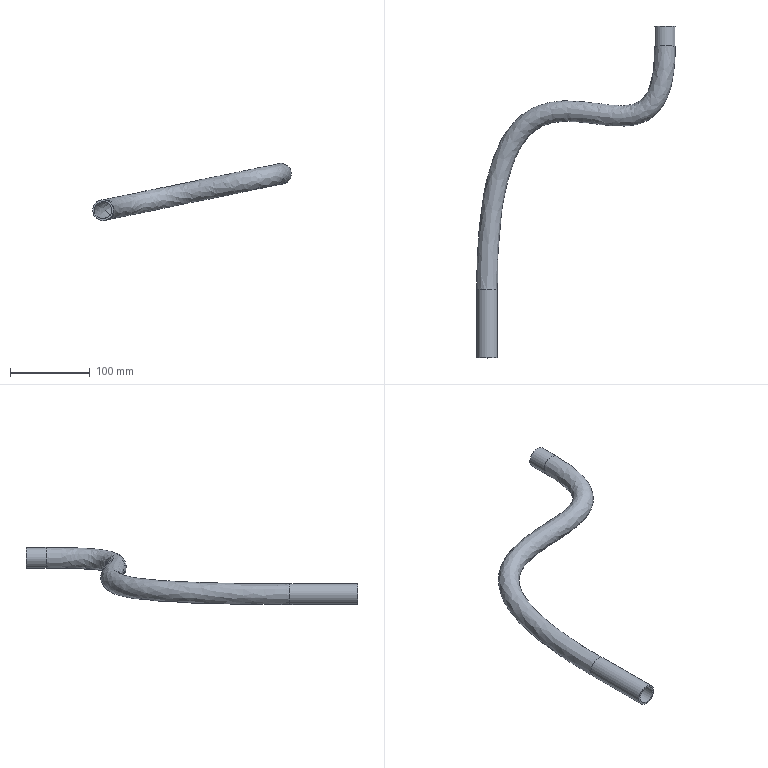Part | STEP file | Part 11^JBJ-F-0000-00 | 1 solid | 8 faces | box 248.297 x 414.992 x 71.5 mm | volume 86273 mm3 | cylinder 4 | spline 2 | plane 2 | commonest cylinder face diameters 22 x2 26 x2